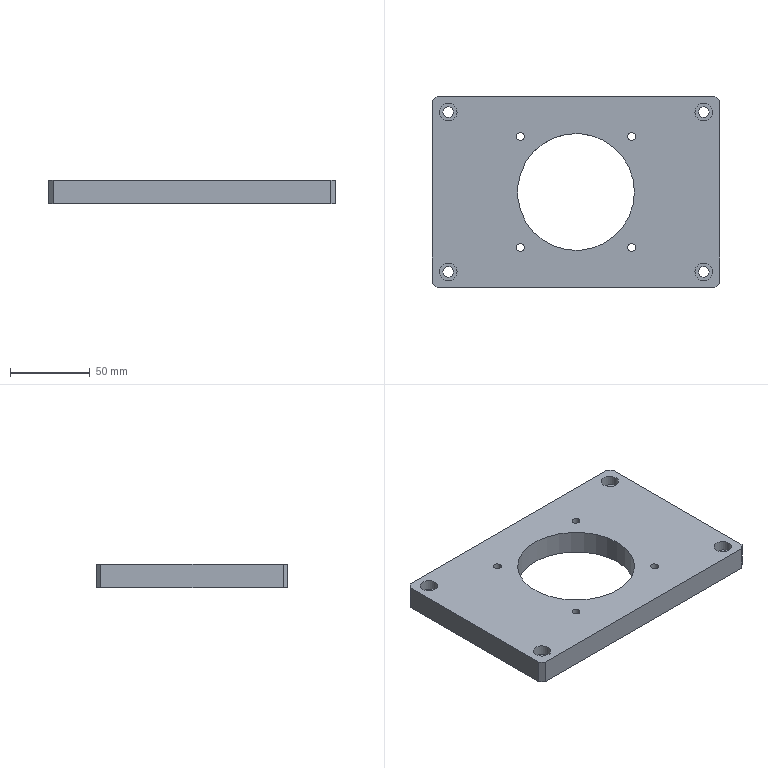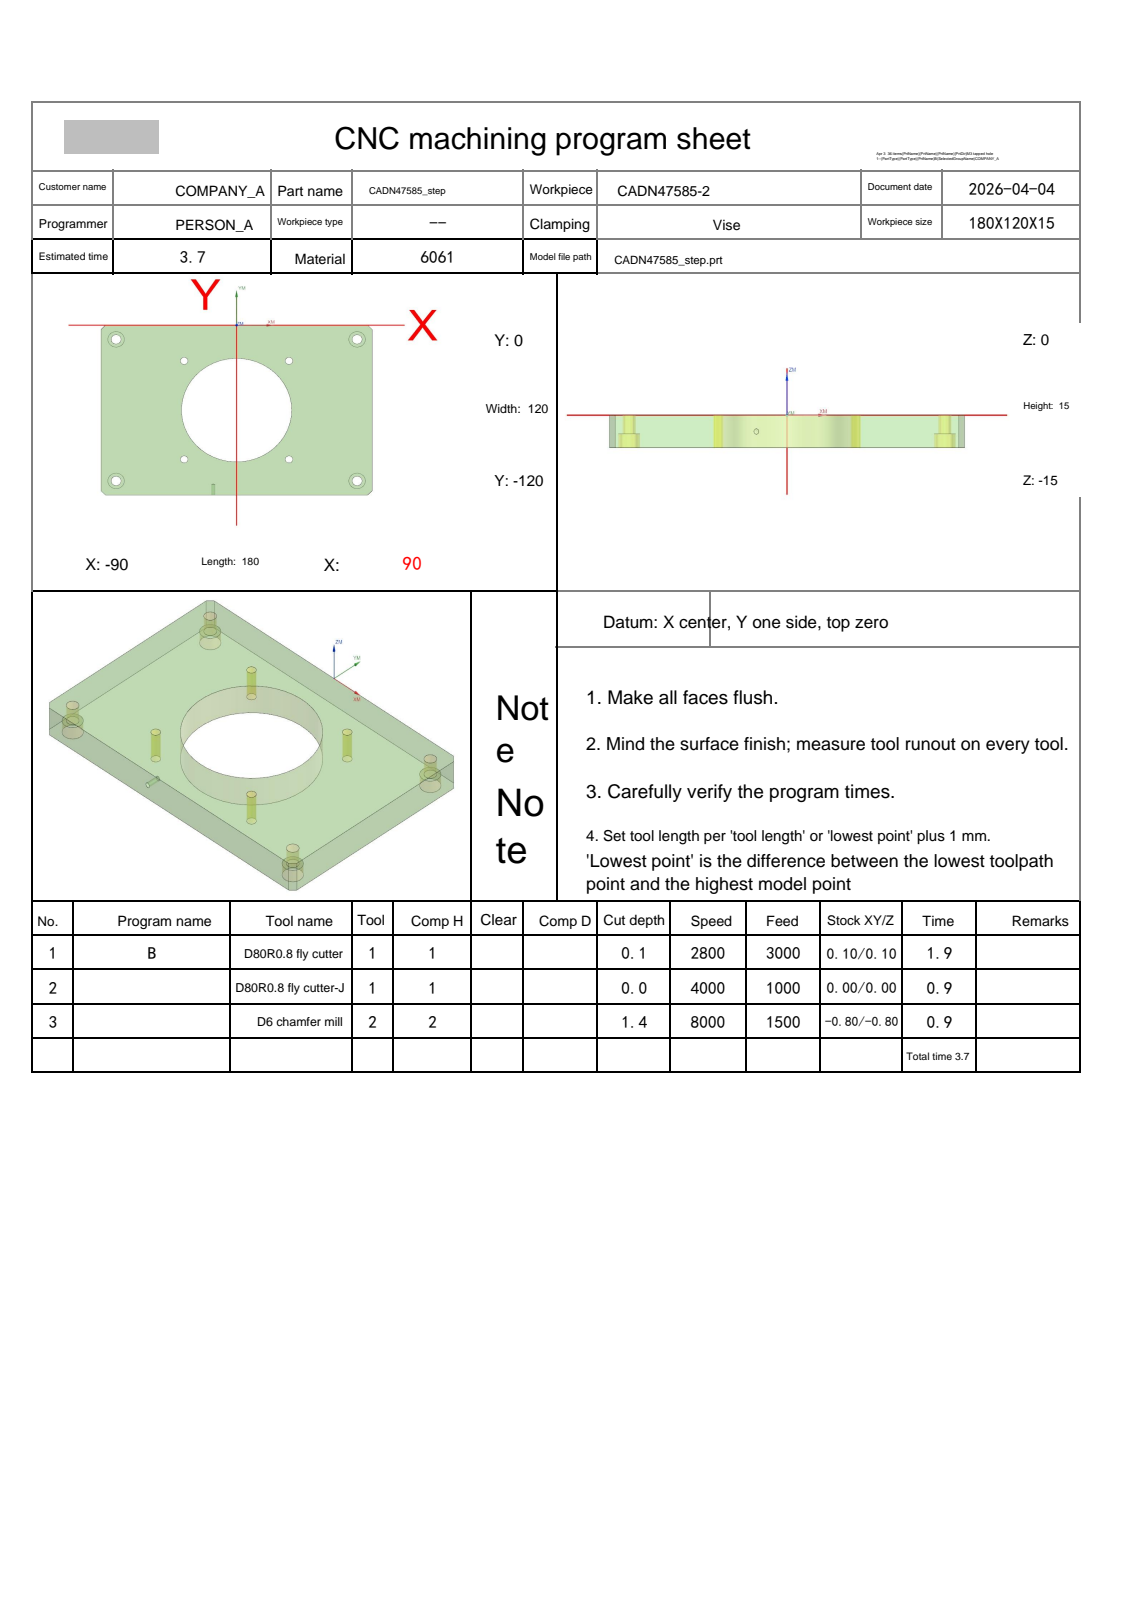NC program | NX | posted by the shop | part box 180 x 120 x 15 mm
Whole program:
%
O0001
(Machine time: 4.20 MIN)
(===Total Tool:2===)
(T1=D80R0.8 fly cutter D=80.  R=0.8  D-  H01 Z=0.    )
(T2=D6 chamfer mill   D=6.   R=0.   D-  H02 Z=-1.4  )
G80 G90 G17 G49 G40
G91 G28 Z0
M01
N1 T01 M06
(D80R0.8 fly cutter  D=80. R=0.8 H=01 ce=0.10 di=0.10)
G00 G90 G54 X142.097 Y-96.097 M03 S2800
G43 H01 Z20.
M08
Z6.011
G01 Z4.011 F3000.
X130.097
X-122.1
G02 X-130.097 Y-88.1 I.003 J8.
G01 Y-39.26
G02 X-122.1 Y-31.263 I8. J-.003
G01 X130.097
X142.097
Z6.011
G00 Y-96.097
Z5.522
G01 Z3.522
X130.097
X-122.1
G02 X-130.097 Y-88.1 I.003 J8.
G01 Y-39.26
G02 X-122.1 Y-31.263 I8. J-.003
G01 X130.097
X142.097
Z5.522
G00 Y-96.097
Z5.033
G01 Z3.033
X130.097
X-122.1
G02 X-130.097 Y-88.1 I.003 J8.
G01 Y-39.26
G02 X-122.1 Y-31.263 I8. J-.003
G01 X130.097
X142.097
Z5.033
G00 Y-96.097
Z4.544
G01 Z2.544
X130.097
X-122.1
G02 X-130.097 Y-88.1 I.003 J8.
G01 Y-39.26
G02 X-122.1 Y-31.263 I8. J-.003
G01 X130.097
X142.097
Z4.544
G00 Y-96.097
Z4.056
G01 Z2.056
X130.097
X-122.1
G02 X-130.097 Y-88.1 I.003 J8.
G01 Y-39.26
G02 X-122.1 Y-31.263 I8. J-.003
G01 X130.097
X142.097
Z4.056
G00 Y-96.097
Z3.567
G01 Z1.567
X130.097
X-122.1
G02 X-130.097 Y-88.1 I.003 J8.
G01 Y-39.26
G02 X-122.1 Y-31.263 I8. J-.003
G01 X130.097
X142.097
Z3.567
G00 Y-96.097
Z3.078
G01 Z1.078
X130.097
X-122.1
G02 X-130.097 Y-88.1 I.003 J8.
G01 Y-39.26
G02 X-122.1 Y-31.263 I8. J-.003
G01 X130.097
X142.097
Z3.078
G00 Y-96.097
Z2.589
G01 Z.589
X130.097
X-122.1
G02 X-130.097 Y-88.1 I.003 J8.
G01 Y-39.26
G02 X-122.1 Y-31.263 I8. J-.003
G01 X130.097
X142.097
Z2.589
G00 Y-96.097
Z2.1
G01 Z.1
X130.097
X-122.1
G02 X-130.097 Y-88.1 I.003 J8.
G01 Y-39.26
G02 X-122.1 Y-31.263 I8. J-.003
G01 X130.097
X142.097
Z2.1
G00 Z20.
G91 G28 Z0.0
M05
M09
G91 G28 Z0.0
M01
N2 T01 M06
(D80R0.8 fly cutter-J  D=80. R=0.8 H=01 ce=0.00 di=0.00)
G00 G90 G54 X141.999 Y-95.999 M03 S4000
G43 H01 Z20.
M08
Z2.
G01 Z0.0 F1000.
X129.999
X-122.799
G02 X-129.999 Y-88.799 I0.0 J7.2
G01 Y-71.68
G02 X-121.999 Y-63.68 I8. J0.0
G01 X122.799
G03 X129.999 Y-56.48 I0.0 J7.2
G01 Y-39.361
G03 X121.999 Y-31.361 I-8. J0.0
G01 X-129.999
X-141.999
Z2.
G00 Z20.
G91 G28 Z0.0
M05
M09
G91 G28 Z0.0
M01
N3 T02 M06
(D6 chamfer mill  D=6. R=0. H=02 ce=-0.80 di=-0.80)
G00 G90 G54 X34.568 Y-24.33 M03 S8000
G43 H02 Z20.
M08
Z-.9
G01 Z-1.4 F600.
X34.4 Y-23.7
G03 X32.9 Y-25.2 I0.0 J-1.5
X34.8 Y-27.1 I1.9 J0.0
X36.7 Y-25.2 I0.0 J1.9
X34.8 Y-23.3 I-1.9 J0.0
X32.9 Y-25.2 I0.0 J-1.9
X34.4 Y-26.7 I1.5 J0.0
G01 X34.568 Y-26.07
Z-.9
G00 Z20.
Y-93.93
Z-.9
G01 Z-1.4
X34.4 Y-93.3
G03 X32.9 Y-94.8 I0.0 J-1.5
X34.8 Y-96.7 I1.9 J0.0
X36.7 Y-94.8 I0.0 J1.9
X34.8 Y-92.9 I-1.9 J0.0
X32.9 Y-94.8 I0.0 J-1.9
X34.4 Y-96.3 I1.5 J0.0
G01 X34.568 Y-95.67
Z-.9
G00 Z20.
X-35.032 Y-93.93
Z-.9
G01 Z-1.4
X-35.2 Y-93.3
G03 X-36.7 Y-94.8 I0.0 J-1.5
X-34.8 Y-96.7 I1.9 J0.0
X-32.9 Y-94.8 I0.0 J1.9
X-34.8 Y-92.9 I-1.9 J0.0
X-36.7 Y-94.8 I0.0 J-1.9
X-35.2 Y-96.3 I1.5 J0.0
G01 X-35.032 Y-95.67
Z-.9
G00 Z20.
Y-24.33
Z-.9
G01 Z-1.4
X-35.2 Y-23.7
G03 X-36.7 Y-25.2 I0.0 J-1.5
X-34.8 Y-27.1 I1.9 J0.0
X-32.9 Y-25.2 I0.0 J1.9
X-34.8 Y-23.3 I-1.9 J0.0
X-36.7 Y-25.2 I0.0 J-1.9
X-35.2 Y-26.7 I1.5 J0.0
G01 X-35.032 Y-26.07
Z-.9
G00 Z20.
G00 G90 X79.493 Y-8.913 M03 S8000
Z20.
Z-.9
G01 Z-1.4 F1200.
X79.3 Y-8.5
G03 X77.8 Y-10. I0.0 J-1.5
X80. Y-12.2 I2.2 J0.0
X82.2 Y-10. I0.0 J2.2
X80. Y-7.8 I-2.2 J0.0
X77.8 Y-10. I0.0 J-2.2
X79.3 Y-11.5 I1.5 J0.0
G01 X79.493 Y-11.087
Z-.9
G00 Z20.
Y-108.913
Z-.9
G01 Z-1.4
X79.3 Y-108.5
G03 X77.8 Y-110. I0.0 J-1.5
X80. Y-112.2 I2.2 J0.0
X82.2 Y-110. I0.0 J2.2
X80. Y-107.8 I-2.2 J0.0
X77.8 Y-110. I0.0 J-2.2
X79.3 Y-111.5 I1.5 J0.0
G01 X79.493 Y-111.087
Z-.9
G00 Z20.
X-80.507 Y-108.913
Z-.9
G01 Z-1.4
X-80.7 Y-108.5
G03 X-82.2 Y-110. I0.0 J-1.5
X-80. Y-112.2 I2.2 J0.0
X-77.8 Y-110. I0.0 J2.2
X-80. Y-107.8 I-2.2 J0.0
X-82.2 Y-110. I0.0 J-2.2
X-80.7 Y-111.5 I1.5 J0.0
G01 X-80.507 Y-111.087
Z-.9
G00 Z20.
Y-8.913
Z-.9
G01 Z-1.4
X-80.7 Y-8.5
G03 X-82.2 Y-10. I0.0 J-1.5
X-80. Y-12.2 I2.2 J0.0
X-77.8 Y-10. I0.0 J2.2
X-80. Y-7.8 I-2.2 J0.0
X-82.2 Y-10. I0.0 J-2.2
X-80.7 Y-11.5 I1.5 J0.0
G01 X-80.507 Y-11.087
Z-.9
G00 Z20.
G00 G90 X78.046 Y.7 M03 S7000
Z20.
Z2.5
G01 X86.876 Z-.714 F1500.
X86.953 Z-.742
X87.16 Y.662 Z-.819
X87.355 Y.581 Z-.895
X87.528 Y.462 Z-.972
X87.583 Y.407 Z-1.
X90.407 Y-2.417
G02 X90.7 Y-3.124 I-.707 J-.707
G01 Y-116.876
G02 X90.407 Y-117.583 I-1. J0.0
G01 X87.583 Y-120.407
G02 X86.876 Y-120.7 I-.707 J.707
G01 X-86.876
G02 X-87.583 Y-120.407 I0.0 J1.
G01 X-90.407 Y-117.583
G02 X-90.7 Y-116.876 I.707 J.707
G01 Y-3.124
G02 X-90.407 Y-2.417 I1. J0.0
G01 X-87.583 Y.407
G02 X-86.876 Y.7 I.707 J-.707
G01 X86.876
G02 X87.583 Y.407 I0.0 J-1.
G01 X87.936 Y.054
Z1.5
G00 Z20.
X34.622 Y-69.502
Z2.5
G01 X34.631 Y-69.471 Z2.488
X34.952 Y-68.208 Z2.014
X35.227 Y-66.935 Z1.54
X35.455 Y-65.652 Z1.066
X35.637 Y-64.362 Z.592
X35.772 Y-63.066 Z.117
X35.86 Y-61.766 Z-.357
X35.9 Y-60.464 Z-.831
Y-60. Z-1.
G03 X0.0 Y-24.1 I-35.9 J0.0
X-35.9 Y-60. I0.0 J-35.9
X0.0 Y-95.9 I35.9 J0.0
X35.9 Y-60. I0.0 J35.9
X35.897 Y-59.5 I-35.9 J0.0
G01 Z1.5
G00 Z20.
M05
M09
G91 G28 Z0.0
G91 G28 Y0.0
M30
%